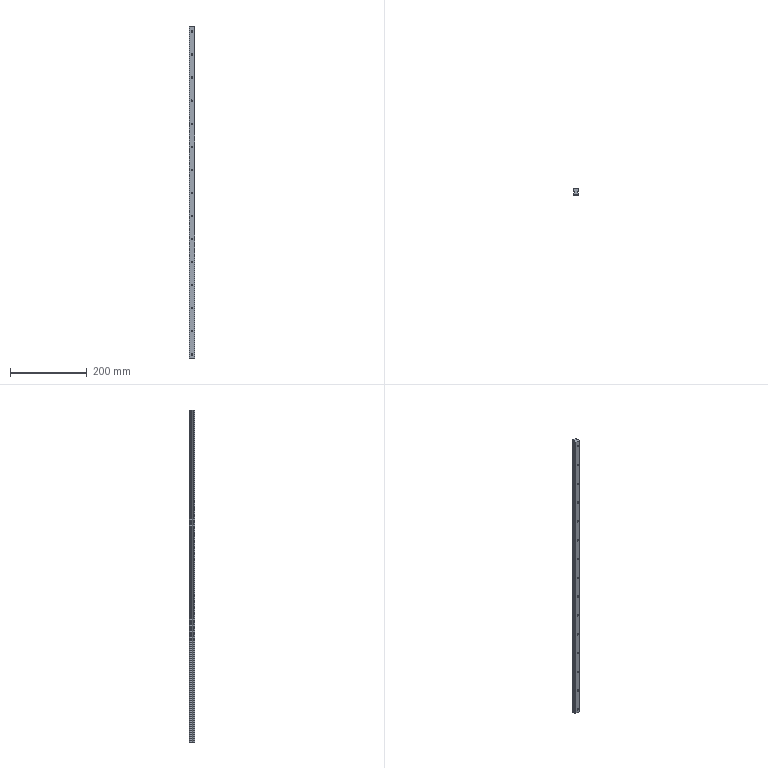Part | STEP file | 11-HGR1511 | 1 solid | 111 faces | box 15 x 15 x 865 mm | volume 159164 mm3 | cylinder 74 | plane 37 | commonest cylinder face diameters 4.5 x30 8 x24 0.8 x8 7.5 x6 3.24 x4 2 x2